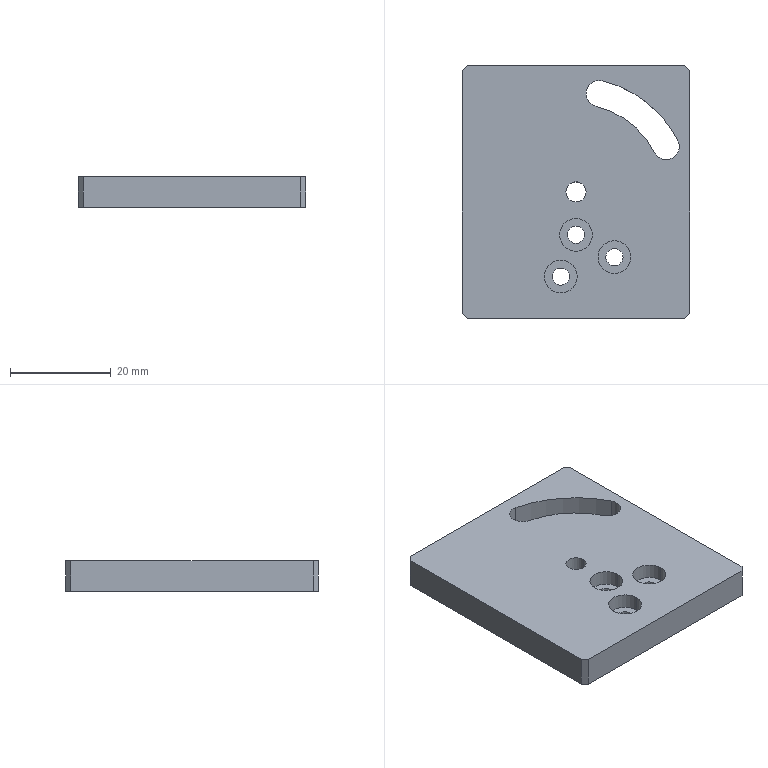Part | NX | features BREP 1 | 1 solid | 32 faces | box 45 x 50 x 6 mm | volume 12360 mm3 | cylinder 19 | plane 13 | commonest cylinder face diameters 3.4 x6 6.5 x6 5.2 x3 4 x2 34.8 x1 45.2 x1
STEP:
#1=CARTESIAN_POINT('',(-3.25,-8.489,3.));
#2=VERTEX_POINT('',#1);
#3=CARTESIAN_POINT('',(3.25,-8.489,3.));
#4=VERTEX_POINT('',#3);
#5=CARTESIAN_POINT('',(0.,-8.489,3.));
#6=DIRECTION('',(0.,0.,1.));
#7=DIRECTION('',(1.,0.,0.));
#8=AXIS2_PLACEMENT_3D('',#5,#6,#7);
#9=CIRCLE('',#8,3.25);
#10=EDGE_CURVE('',#2,#4,#9,.T.);
#11=ORIENTED_EDGE('',*,*,#10,.F.);
#12=CARTESIAN_POINT('',(-3.25,-8.489,6.));
#13=VERTEX_POINT('',#12);
#14=CARTESIAN_POINT('',(-3.25,-8.489,6.));
#15=DIRECTION('',(0.,0.,1.));
#16=VECTOR('',#15,1000.);
#17=LINE('',#14,#16);
#18=EDGE_CURVE('',#13,#2,#17,.F.);
#19=ORIENTED_EDGE('',*,*,#18,.F.);
#20=CARTESIAN_POINT('',(3.25,-8.489,6.));
#21=VERTEX_POINT('',#20);
#22=CARTESIAN_POINT('',(0.,-8.489,6.));
#23=DIRECTION('',(0.,0.,1.));
#24=DIRECTION('',(1.,0.,0.));
#25=AXIS2_PLACEMENT_3D('',#22,#23,#24);
#26=CIRCLE('',#25,3.25);
#27=EDGE_CURVE('',#13,#21,#26,.T.);
#28=ORIENTED_EDGE('',*,*,#27,.T.);
#29=CARTESIAN_POINT('',(3.25,-8.489,6.));
#30=DIRECTION('',(0.,0.,1.));
#31=VECTOR('',#30,1000.);
#32=LINE('',#29,#31);
#33=EDGE_CURVE('',#21,#4,#32,.F.);
#34=ORIENTED_EDGE('',*,*,#33,.T.);
#35=EDGE_LOOP('',(#11,#19,#28,#34));
#36=FACE_BOUND('',#35,.T.);
#37=CARTESIAN_POINT('',(0.,-8.489,6.));
#38=DIRECTION('',(0.,0.,1.));
#39=DIRECTION('',(1.,0.,0.));
#40=AXIS2_PLACEMENT_3D('',#37,#38,#39);
#41=CYLINDRICAL_SURFACE('',#40,3.25);
#42=ADVANCED_FACE('',(#36),#41,.F.);
#43=CARTESIAN_POINT('',(-1.7,-8.489,0.));
#44=VERTEX_POINT('',#43);
#45=CARTESIAN_POINT('',(1.7,-8.489,0.));
#46=VERTEX_POINT('',#45);
#47=CARTESIAN_POINT('',(0.,-8.489,0.));
#48=DIRECTION('',(0.,0.,1.));
#49=DIRECTION('',(1.,0.,0.));
#50=AXIS2_PLACEMENT_3D('',#47,#48,#49);
#51=CIRCLE('',#50,1.7);
#52=EDGE_CURVE('',#44,#46,#51,.T.);
#53=ORIENTED_EDGE('',*,*,#52,.F.);
#54=CARTESIAN_POINT('',(-1.7,-8.489,3.));
#55=VERTEX_POINT('',#54);
#56=CARTESIAN_POINT('',(-1.7,-8.489,6.));
#57=DIRECTION('',(0.,0.,1.));
#58=VECTOR('',#57,1000.);
#59=LINE('',#56,#58);
#60=EDGE_CURVE('',#55,#44,#59,.F.);
#61=ORIENTED_EDGE('',*,*,#60,.F.);
#62=CARTESIAN_POINT('',(1.7,-8.489,3.));
#63=VERTEX_POINT('',#62);
#64=CARTESIAN_POINT('',(0.,-8.489,3.));
#65=DIRECTION('',(0.,0.,1.));
#66=DIRECTION('',(1.,0.,0.));
#67=AXIS2_PLACEMENT_3D('',#64,#65,#66);
#68=CIRCLE('',#67,1.7);
#69=EDGE_CURVE('',#55,#63,#68,.T.);
#70=ORIENTED_EDGE('',*,*,#69,.T.);
#71=CARTESIAN_POINT('',(1.7,-8.489,6.));
#72=DIRECTION('',(0.,0.,1.));
#73=VECTOR('',#72,1000.);
#74=LINE('',#71,#73);
#75=EDGE_CURVE('',#63,#46,#74,.F.);
#76=ORIENTED_EDGE('',*,*,#75,.T.);
#77=EDGE_LOOP('',(#53,#61,#70,#76));
#78=FACE_BOUND('',#77,.T.);
#79=CARTESIAN_POINT('',(0.,-8.489,6.));
#80=DIRECTION('',(0.,0.,1.));
#81=DIRECTION('',(1.,0.,0.));
#82=AXIS2_PLACEMENT_3D('',#79,#80,#81);
#83=CYLINDRICAL_SURFACE('',#82,1.7);
#84=ADVANCED_FACE('',(#78),#83,.F.);
#85=CARTESIAN_POINT('',(-6.26,-16.759,3.));
#86=VERTEX_POINT('',#85);
#87=CARTESIAN_POINT('',(0.2402,-16.759,3.));
#88=VERTEX_POINT('',#87);
#89=CARTESIAN_POINT('',(-3.01,-16.759,3.));
#90=DIRECTION('',(0.,0.,1.));
#91=DIRECTION('',(1.,0.,0.));
#92=AXIS2_PLACEMENT_3D('',#89,#90,#91);
#93=CIRCLE('',#92,3.25);
#94=EDGE_CURVE('',#86,#88,#93,.T.);
#95=ORIENTED_EDGE('',*,*,#94,.F.);
#96=CARTESIAN_POINT('',(-6.26,-16.759,6.));
#97=VERTEX_POINT('',#96);
#98=CARTESIAN_POINT('',(-6.26,-16.759,6.));
#99=DIRECTION('',(0.,0.,1.));
#100=VECTOR('',#99,1000.);
#101=LINE('',#98,#100);
#102=EDGE_CURVE('',#97,#86,#101,.F.);
#103=ORIENTED_EDGE('',*,*,#102,.F.);
#104=CARTESIAN_POINT('',(0.2402,-16.759,6.));
#105=VERTEX_POINT('',#104);
#106=CARTESIAN_POINT('',(-3.01,-16.759,6.));
#107=DIRECTION('',(0.,0.,1.));
#108=DIRECTION('',(1.,0.,0.));
#109=AXIS2_PLACEMENT_3D('',#106,#107,#108);
#110=CIRCLE('',#109,3.25);
#111=EDGE_CURVE('',#97,#105,#110,.T.);
#112=ORIENTED_EDGE('',*,*,#111,.T.);
#113=CARTESIAN_POINT('',(0.2402,-16.759,6.));
#114=DIRECTION('',(0.,0.,1.));
#115=VECTOR('',#114,1000.);
#116=LINE('',#113,#115);
#117=EDGE_CURVE('',#105,#88,#116,.F.);
#118=ORIENTED_EDGE('',*,*,#117,.T.);
#119=EDGE_LOOP('',(#95,#103,#112,#118));
#120=FACE_BOUND('',#119,.T.);
#121=CARTESIAN_POINT('',(-3.01,-16.759,6.));
#122=DIRECTION('',(0.,0.,1.));
#123=DIRECTION('',(1.,0.,0.));
#124=AXIS2_PLACEMENT_3D('',#121,#122,#123);
#125=CYLINDRICAL_SURFACE('',#124,3.25);
#126=ADVANCED_FACE('',(#120),#125,.F.);
#127=CARTESIAN_POINT('',(-4.71,-16.759,0.));
#128=VERTEX_POINT('',#127);
#129=CARTESIAN_POINT('',(-1.31,-16.759,0.));
#130=VERTEX_POINT('',#129);
#131=CARTESIAN_POINT('',(-3.01,-16.759,0.));
#132=DIRECTION('',(0.,0.,1.));
#133=DIRECTION('',(1.,0.,0.));
#134=AXIS2_PLACEMENT_3D('',#131,#132,#133);
#135=CIRCLE('',#134,1.7);
#136=EDGE_CURVE('',#128,#130,#135,.T.);
#137=ORIENTED_EDGE('',*,*,#136,.F.);
#138=CARTESIAN_POINT('',(-4.71,-16.759,3.));
#139=VERTEX_POINT('',#138);
#140=CARTESIAN_POINT('',(-4.71,-16.759,6.));
#141=DIRECTION('',(0.,0.,1.));
#142=VECTOR('',#141,1000.);
#143=LINE('',#140,#142);
#144=EDGE_CURVE('',#139,#128,#143,.F.);
#145=ORIENTED_EDGE('',*,*,#144,.F.);
#146=CARTESIAN_POINT('',(-1.31,-16.759,3.));
#147=VERTEX_POINT('',#146);
#148=CARTESIAN_POINT('',(-3.01,-16.759,3.));
#149=DIRECTION('',(0.,0.,1.));
#150=DIRECTION('',(1.,0.,0.));
#151=AXIS2_PLACEMENT_3D('',#148,#149,#150);
#152=CIRCLE('',#151,1.7);
#153=EDGE_CURVE('',#139,#147,#152,.T.);
#154=ORIENTED_EDGE('',*,*,#153,.T.);
#155=CARTESIAN_POINT('',(-1.31,-16.759,6.));
#156=DIRECTION('',(0.,0.,1.));
#157=VECTOR('',#156,1000.);
#158=LINE('',#155,#157);
#159=EDGE_CURVE('',#147,#130,#158,.F.);
#160=ORIENTED_EDGE('',*,*,#159,.T.);
#161=EDGE_LOOP('',(#137,#145,#154,#160));
#162=FACE_BOUND('',#161,.T.);
#163=CARTESIAN_POINT('',(-3.01,-16.759,6.));
#164=DIRECTION('',(0.,0.,1.));
#165=DIRECTION('',(1.,0.,0.));
#166=AXIS2_PLACEMENT_3D('',#163,#164,#165);
#167=CYLINDRICAL_SURFACE('',#166,1.7);
#168=ADVANCED_FACE('',(#162),#167,.F.);
#169=CARTESIAN_POINT('',(4.362,-12.904,3.));
#170=VERTEX_POINT('',#169);
#171=CARTESIAN_POINT('',(10.862,-12.904,3.));
#172=VERTEX_POINT('',#171);
#173=CARTESIAN_POINT('',(7.612,-12.904,3.));
#174=DIRECTION('',(0.,0.,1.));
#175=DIRECTION('',(1.,0.,0.));
#176=AXIS2_PLACEMENT_3D('',#173,#174,#175);
#177=CIRCLE('',#176,3.25);
#178=EDGE_CURVE('',#170,#172,#177,.T.);
#179=ORIENTED_EDGE('',*,*,#178,.F.);
#180=CARTESIAN_POINT('',(4.362,-12.904,6.));
#181=VERTEX_POINT('',#180);
#182=CARTESIAN_POINT('',(4.362,-12.904,6.));
#183=DIRECTION('',(0.,0.,1.));
#184=VECTOR('',#183,1000.);
#185=LINE('',#182,#184);
#186=EDGE_CURVE('',#181,#170,#185,.F.);
#187=ORIENTED_EDGE('',*,*,#186,.F.);
#188=CARTESIAN_POINT('',(10.862,-12.904,6.));
#189=VERTEX_POINT('',#188);
#190=CARTESIAN_POINT('',(7.612,-12.904,6.));
#191=DIRECTION('',(0.,0.,1.));
#192=DIRECTION('',(1.,0.,0.));
#193=AXIS2_PLACEMENT_3D('',#190,#191,#192);
#194=CIRCLE('',#193,3.25);
#195=EDGE_CURVE('',#181,#189,#194,.T.);
#196=ORIENTED_EDGE('',*,*,#195,.T.);
#197=CARTESIAN_POINT('',(10.862,-12.904,6.));
#198=DIRECTION('',(0.,0.,1.));
#199=VECTOR('',#198,1000.);
#200=LINE('',#197,#199);
#201=EDGE_CURVE('',#189,#172,#200,.F.);
#202=ORIENTED_EDGE('',*,*,#201,.T.);
#203=EDGE_LOOP('',(#179,#187,#196,#202));
#204=FACE_BOUND('',#203,.T.);
#205=CARTESIAN_POINT('',(7.612,-12.904,6.));
#206=DIRECTION('',(0.,0.,1.));
#207=DIRECTION('',(1.,0.,0.));
#208=AXIS2_PLACEMENT_3D('',#205,#206,#207);
#209=CYLINDRICAL_SURFACE('',#208,3.25);
#210=ADVANCED_FACE('',(#204),#209,.F.);
#211=CARTESIAN_POINT('',(5.912,-12.904,0.));
#212=VERTEX_POINT('',#211);
#213=CARTESIAN_POINT('',(9.312,-12.904,0.));
#214=VERTEX_POINT('',#213);
#215=CARTESIAN_POINT('',(7.612,-12.904,0.));
#216=DIRECTION('',(0.,0.,1.));
#217=DIRECTION('',(1.,0.,0.));
#218=AXIS2_PLACEMENT_3D('',#215,#216,#217);
#219=CIRCLE('',#218,1.7);
#220=EDGE_CURVE('',#212,#214,#219,.T.);
#221=ORIENTED_EDGE('',*,*,#220,.F.);
#222=CARTESIAN_POINT('',(5.912,-12.904,3.));
#223=VERTEX_POINT('',#222);
#224=CARTESIAN_POINT('',(5.912,-12.904,6.));
#225=DIRECTION('',(0.,0.,1.));
#226=VECTOR('',#225,1000.);
#227=LINE('',#224,#226);
#228=EDGE_CURVE('',#223,#212,#227,.F.);
#229=ORIENTED_EDGE('',*,*,#228,.F.);
#230=CARTESIAN_POINT('',(9.312,-12.904,3.));
#231=VERTEX_POINT('',#230);
#232=CARTESIAN_POINT('',(7.612,-12.904,3.));
#233=DIRECTION('',(0.,0.,1.));
#234=DIRECTION('',(1.,0.,0.));
#235=AXIS2_PLACEMENT_3D('',#232,#233,#234);
#236=CIRCLE('',#235,1.7);
#237=EDGE_CURVE('',#223,#231,#236,.T.);
#238=ORIENTED_EDGE('',*,*,#237,.T.);
#239=CARTESIAN_POINT('',(9.312,-12.904,6.));
#240=DIRECTION('',(0.,0.,1.));
#241=VECTOR('',#240,1000.);
#242=LINE('',#239,#241);
#243=EDGE_CURVE('',#231,#214,#242,.F.);
#244=ORIENTED_EDGE('',*,*,#243,.T.);
#245=EDGE_LOOP('',(#221,#229,#238,#244));
#246=FACE_BOUND('',#245,.T.);
#247=CARTESIAN_POINT('',(7.612,-12.904,6.));
#248=DIRECTION('',(0.,0.,1.));
#249=DIRECTION('',(1.,0.,0.));
#250=AXIS2_PLACEMENT_3D('',#247,#248,#249);
#251=CYLINDRICAL_SURFACE('',#250,1.7);
#252=ADVANCED_FACE('',(#246),#251,.F.);
#253=CARTESIAN_POINT('',(5.182,21.998,6.));
#254=VERTEX_POINT('',#253);
#255=CARTESIAN_POINT('',(1.986,19.467,6.));
#256=VERTEX_POINT('',#255);
#257=CARTESIAN_POINT('',(4.586,19.467,6.));
#258=DIRECTION('',(0.,0.,1.));
#259=DIRECTION('',(1.,0.,0.));
#260=AXIS2_PLACEMENT_3D('',#257,#258,#259);
#261=CIRCLE('',#260,2.6);
#262=EDGE_CURVE('',#254,#256,#261,.T.);
#263=ORIENTED_EDGE('',*,*,#262,.T.);
#264=CARTESIAN_POINT('',(1.986,19.467,0.));
#265=VERTEX_POINT('',#264);
#266=CARTESIAN_POINT('',(1.986,19.467,10.));
#267=DIRECTION('',(0.,0.,-1.));
#268=VECTOR('',#267,1000.);
#269=LINE('',#266,#268);
#270=EDGE_CURVE('',#256,#265,#269,.T.);
#271=ORIENTED_EDGE('',*,*,#270,.T.);
#272=CARTESIAN_POINT('',(5.182,21.998,0.));
#273=VERTEX_POINT('',#272);
#274=CARTESIAN_POINT('',(4.586,19.467,0.));
#275=DIRECTION('',(0.,0.,-1.));
#276=DIRECTION('',(-1.,0.,0.));
#277=AXIS2_PLACEMENT_3D('',#274,#275,#276);
#278=CIRCLE('',#277,2.6);
#279=EDGE_CURVE('',#265,#273,#278,.T.);
#280=ORIENTED_EDGE('',*,*,#279,.T.);
#281=CARTESIAN_POINT('',(5.182,21.998,10.));
#282=DIRECTION('',(0.,0.,-1.));
#283=VECTOR('',#282,1000.);
#284=LINE('',#281,#283);
#285=EDGE_CURVE('',#254,#273,#284,.T.);
#286=ORIENTED_EDGE('',*,*,#285,.F.);
#287=EDGE_LOOP('',(#263,#271,#280,#286));
#288=FACE_BOUND('',#287,.T.);
#289=CARTESIAN_POINT('',(4.586,19.467,10.));
#290=DIRECTION('',(0.,0.,-1.));
#291=DIRECTION('',(-1.,0.,0.));
#292=AXIS2_PLACEMENT_3D('',#289,#290,#291);
#293=CYLINDRICAL_SURFACE('',#292,2.6);
#294=ADVANCED_FACE('',(#288),#293,.F.);
#295=CARTESIAN_POINT('',(-2.,0.,6.));
#296=VERTEX_POINT('',#295);
#297=CARTESIAN_POINT('',(2.,0.,6.));
#298=VERTEX_POINT('',#297);
#299=CARTESIAN_POINT('',(0.,0.,6.));
#300=DIRECTION('',(0.,0.,1.));
#301=DIRECTION('',(1.,0.,0.));
#302=AXIS2_PLACEMENT_3D('',#299,#300,#301);
#303=CIRCLE('',#302,2.);
#304=EDGE_CURVE('',#296,#298,#303,.T.);
#305=ORIENTED_EDGE('',*,*,#304,.T.);
#306=CARTESIAN_POINT('',(2.,0.,0.));
#307=VERTEX_POINT('',#306);
#308=CARTESIAN_POINT('',(2.,0.,10.));
#309=DIRECTION('',(0.,0.,-1.));
#310=VECTOR('',#309,1000.);
#311=LINE('',#308,#310);
#312=EDGE_CURVE('',#298,#307,#311,.T.);
#313=ORIENTED_EDGE('',*,*,#312,.T.);
#314=CARTESIAN_POINT('',(-2.,0.,0.));
#315=VERTEX_POINT('',#314);
#316=CARTESIAN_POINT('',(0.,0.,0.));
#317=DIRECTION('',(0.,0.,-1.));
#318=DIRECTION('',(-1.,0.,0.));
#319=AXIS2_PLACEMENT_3D('',#316,#317,#318);
#320=CIRCLE('',#319,2.);
#321=EDGE_CURVE('',#307,#315,#320,.T.);
#322=ORIENTED_EDGE('',*,*,#321,.T.);
#323=CARTESIAN_POINT('',(-2.,0.,10.));
#324=DIRECTION('',(0.,0.,-1.));
#325=VECTOR('',#324,1000.);
#326=LINE('',#323,#325);
#327=EDGE_CURVE('',#296,#315,#326,.T.);
#328=ORIENTED_EDGE('',*,*,#327,.F.);
#329=EDGE_LOOP('',(#305,#313,#322,#328));
#330=FACE_BOUND('',#329,.T.);
#331=CARTESIAN_POINT('',(0.,0.,10.));
#332=DIRECTION('',(0.,0.,-1.));
#333=DIRECTION('',(-1.,0.,0.));
#334=AXIS2_PLACEMENT_3D('',#331,#332,#333);
#335=CYLINDRICAL_SURFACE('',#334,2.);
#336=ADVANCED_FACE('',(#330),#335,.F.);
#337=CARTESIAN_POINT('',(22.5,-24.,6.));
#338=VERTEX_POINT('',#337);
#339=CARTESIAN_POINT('',(22.5,24.,6.));
#340=VERTEX_POINT('',#339);
#341=CARTESIAN_POINT('',(22.5,25.,6.));
#342=DIRECTION('',(0.,1.,0.));
#343=VECTOR('',#342,1000.);
#344=LINE('',#341,#343);
#345=EDGE_CURVE('',#338,#340,#344,.T.);
#346=ORIENTED_EDGE('',*,*,#345,.F.);
#347=CARTESIAN_POINT('',(22.5,-24.,0.));
#348=VERTEX_POINT('',#347);
#349=CARTESIAN_POINT('',(22.5,-24.,6.));
#350=DIRECTION('',(0.,0.,-1.));
#351=VECTOR('',#350,1000.);
#352=LINE('',#349,#351);
#353=EDGE_CURVE('',#338,#348,#352,.T.);
#354=ORIENTED_EDGE('',*,*,#353,.T.);
#355=CARTESIAN_POINT('',(22.5,24.,0.));
#356=VERTEX_POINT('',#355);
#357=CARTESIAN_POINT('',(22.5,25.,0.));
#358=DIRECTION('',(0.,1.,0.));
#359=VECTOR('',#358,1000.);
#360=LINE('',#357,#359);
#361=EDGE_CURVE('',#348,#356,#360,.T.);
#362=ORIENTED_EDGE('',*,*,#361,.T.);
#363=CARTESIAN_POINT('',(22.5,24.,6.));
#364=DIRECTION('',(0.,0.,1.));
#365=VECTOR('',#364,1000.);
#366=LINE('',#363,#365);
#367=EDGE_CURVE('',#356,#340,#366,.T.);
#368=ORIENTED_EDGE('',*,*,#367,.T.);
#369=EDGE_LOOP('',(#346,#354,#362,#368));
#370=FACE_BOUND('',#369,.T.);
#371=CARTESIAN_POINT('',(22.5,25.,6.));
#372=DIRECTION('',(-1.,0.,0.));
#373=DIRECTION('',(0.,1.,0.));
#374=AXIS2_PLACEMENT_3D('',#371,#372,#373);
#375=PLANE('',#374);
#376=ADVANCED_FACE('',(#370),#375,.F.);
#377=CARTESIAN_POINT('',(21.5,25.,0.));
#378=VERTEX_POINT('',#377);
#379=CARTESIAN_POINT('',(-21.5,25.,0.));
#380=VERTEX_POINT('',#379);
#381=CARTESIAN_POINT('',(-22.5,25.,0.));
#382=DIRECTION('',(-1.,0.,0.));
#383=VECTOR('',#382,1000.);
#384=LINE('',#381,#383);
#385=EDGE_CURVE('',#378,#380,#384,.T.);
#386=ORIENTED_EDGE('',*,*,#385,.T.);
#387=CARTESIAN_POINT('',(-21.5,25.,6.));
#388=VERTEX_POINT('',#387);
#389=CARTESIAN_POINT('',(-21.5,25.,6.));
#390=DIRECTION('',(0.,0.,1.));
#391=VECTOR('',#390,1000.);
#392=LINE('',#389,#391);
#393=EDGE_CURVE('',#380,#388,#392,.T.);
#394=ORIENTED_EDGE('',*,*,#393,.T.);
#395=CARTESIAN_POINT('',(21.5,25.,6.));
#396=VERTEX_POINT('',#395);
#397=CARTESIAN_POINT('',(-22.5,25.,6.));
#398=DIRECTION('',(-1.,0.,0.));
#399=VECTOR('',#398,1000.);
#400=LINE('',#397,#399);
#401=EDGE_CURVE('',#396,#388,#400,.T.);
#402=ORIENTED_EDGE('',*,*,#401,.F.);
#403=CARTESIAN_POINT('',(21.5,25.,6.));
#404=DIRECTION('',(0.,0.,-1.));
#405=VECTOR('',#404,1000.);
#406=LINE('',#403,#405);
#407=EDGE_CURVE('',#396,#378,#406,.T.);
#408=ORIENTED_EDGE('',*,*,#407,.T.);
#409=EDGE_LOOP('',(#386,#394,#402,#408));
#410=FACE_BOUND('',#409,.T.);
#411=CARTESIAN_POINT('',(-22.5,25.,6.));
#412=DIRECTION('',(0.,-1.,0.));
#413=DIRECTION('',(0.,0.,-1.));
#414=AXIS2_PLACEMENT_3D('',#411,#412,#413);
#415=PLANE('',#414);
#416=ADVANCED_FACE('',(#410),#415,.F.);
#417=CARTESIAN_POINT('',(-22.5,24.,0.));
#418=VERTEX_POINT('',#417);
#419=CARTESIAN_POINT('',(-22.5,-24.,0.));
#420=VERTEX_POINT('',#419);
#421=CARTESIAN_POINT('',(-22.5,25.,0.));
#422=DIRECTION('',(0.,-1.,0.));
#423=VECTOR('',#422,1000.);
#424=LINE('',#421,#423);
#425=EDGE_CURVE('',#418,#420,#424,.T.);
#426=ORIENTED_EDGE('',*,*,#425,.T.);
#427=CARTESIAN_POINT('',(-22.5,-24.,6.));
#428=VERTEX_POINT('',#427);
#429=CARTESIAN_POINT('',(-22.5,-24.,6.));
#430=DIRECTION('',(0.,0.,1.));
#431=VECTOR('',#430,1000.);
#432=LINE('',#429,#431);
#433=EDGE_CURVE('',#420,#428,#432,.T.);
#434=ORIENTED_EDGE('',*,*,#433,.T.);
#435=CARTESIAN_POINT('',(-22.5,24.,6.));
#436=VERTEX_POINT('',#435);
#437=CARTESIAN_POINT('',(-22.5,25.,6.));
#438=DIRECTION('',(0.,-1.,0.));
#439=VECTOR('',#438,1000.);
#440=LINE('',#437,#439);
#441=EDGE_CURVE('',#436,#428,#440,.T.);
#442=ORIENTED_EDGE('',*,*,#441,.F.);
#443=CARTESIAN_POINT('',(-22.5,24.,6.));
#444=DIRECTION('',(0.,0.,-1.));
#445=VECTOR('',#444,1000.);
#446=LINE('',#443,#445);
#447=EDGE_CURVE('',#436,#418,#446,.T.);
#448=ORIENTED_EDGE('',*,*,#447,.T.);
#449=EDGE_LOOP('',(#426,#434,#442,#448));
#450=FACE_BOUND('',#449,.T.);
#451=CARTESIAN_POINT('',(-22.5,25.,6.));
#452=DIRECTION('',(1.,0.,0.));
#453=DIRECTION('',(0.,1.,0.));
#454=AXIS2_PLACEMENT_3D('',#451,#452,#453);
#455=PLANE('',#454);
#456=ADVANCED_FACE('',(#450),#455,.F.);
#457=CARTESIAN_POINT('',(-21.5,-25.,6.));
#458=VERTEX_POINT('',#457);
#459=CARTESIAN_POINT('',(21.5,-25.,6.));
#460=VERTEX_POINT('',#459);
#461=CARTESIAN_POINT('',(-22.5,-25.,6.));
#462=DIRECTION('',(1.,0.,0.));
#463=VECTOR('',#462,1000.);
#464=LINE('',#461,#463);
#465=EDGE_CURVE('',#458,#460,#464,.T.);
#466=ORIENTED_EDGE('',*,*,#465,.F.);
#467=CARTESIAN_POINT('',(-21.5,-25.,0.));
#468=VERTEX_POINT('',#467);
#469=CARTESIAN_POINT('',(-21.5,-25.,6.));
#470=DIRECTION('',(0.,0.,-1.));
#471=VECTOR('',#470,1000.);
#472=LINE('',#469,#471);
#473=EDGE_CURVE('',#458,#468,#472,.T.);
#474=ORIENTED_EDGE('',*,*,#473,.T.);
#475=CARTESIAN_POINT('',(21.5,-25.,0.));
#476=VERTEX_POINT('',#475);
#477=CARTESIAN_POINT('',(-22.5,-25.,0.));
#478=DIRECTION('',(1.,0.,0.));
#479=VECTOR('',#478,1000.);
#480=LINE('',#477,#479);
#481=EDGE_CURVE('',#468,#476,#480,.T.);
#482=ORIENTED_EDGE('',*,*,#481,.T.);
#483=CARTESIAN_POINT('',(21.5,-25.,6.));
#484=DIRECTION('',(0.,0.,1.));
#485=VECTOR('',#484,1000.);
#486=LINE('',#483,#485);
#487=EDGE_CURVE('',#476,#460,#486,.T.);
#488=ORIENTED_EDGE('',*,*,#487,.T.);
#489=EDGE_LOOP('',(#466,#474,#482,#488));
#490=FACE_BOUND('',#489,.T.);
#491=CARTESIAN_POINT('',(-22.5,-25.,6.));
#492=DIRECTION('',(0.,1.,0.));
#493=DIRECTION('',(1.,0.,0.));
#494=AXIS2_PLACEMENT_3D('',#491,#492,#493);
#495=PLANE('',#494);
#496=ADVANCED_FACE('',(#490),#495,.F.);
#497=ORIENTED_EDGE('',*,*,#441,.T.);
#498=CARTESIAN_POINT('',(-23.25,-23.25,6.));
#499=DIRECTION('',(0.7071,-0.7071,0.));
#500=VECTOR('',#499,1000.);
#501=LINE('',#498,#500);
#502=EDGE_CURVE('',#428,#458,#501,.T.);
#503=ORIENTED_EDGE('',*,*,#502,.T.);
#504=ORIENTED_EDGE('',*,*,#465,.T.);
#505=CARTESIAN_POINT('',(23.25,-23.25,6.));
#506=DIRECTION('',(0.7071,0.7071,0.));
#507=VECTOR('',#506,1000.);
#508=LINE('',#505,#507);
#509=EDGE_CURVE('',#460,#338,#508,.T.);
#510=ORIENTED_EDGE('',*,*,#509,.T.);
#511=ORIENTED_EDGE('',*,*,#345,.T.);
#512=CARTESIAN_POINT('',(23.25,23.25,6.));
#513=DIRECTION('',(-0.7071,0.7071,0.));
#514=VECTOR('',#513,1000.);
#515=LINE('',#512,#514);
#516=EDGE_CURVE('',#340,#396,#515,.T.);
#517=ORIENTED_EDGE('',*,*,#516,.T.);
#518=ORIENTED_EDGE('',*,*,#401,.T.);
#519=CARTESIAN_POINT('',(-23.25,23.25,6.));
#520=DIRECTION('',(-0.7071,-0.7071,0.));
#521=VECTOR('',#520,1000.);
#522=LINE('',#519,#521);
#523=EDGE_CURVE('',#388,#436,#522,.T.);
#524=ORIENTED_EDGE('',*,*,#523,.T.);
#525=EDGE_LOOP('',(#497,#503,#504,#510,#511,#517,#518,#524));
#526=FACE_BOUND('',#525,.T.);
#527=CARTESIAN_POINT('',(0.,-8.489,6.));
#528=DIRECTION('',(0.,0.,1.));
#529=DIRECTION('',(1.,0.,0.));
#530=AXIS2_PLACEMENT_3D('',#527,#528,#529);
#531=CIRCLE('',#530,3.25);
#532=EDGE_CURVE('',#21,#13,#531,.T.);
#533=ORIENTED_EDGE('',*,*,#532,.F.);
#534=ORIENTED_EDGE('',*,*,#27,.F.);
#535=EDGE_LOOP('',(#533,#534));
#536=FACE_BOUND('',#535,.T.);
#537=CARTESIAN_POINT('',(-3.01,-16.759,6.));
#538=DIRECTION('',(0.,0.,1.));
#539=DIRECTION('',(1.,0.,0.));
#540=AXIS2_PLACEMENT_3D('',#537,#538,#539);
#541=CIRCLE('',#540,3.25);
#542=EDGE_CURVE('',#105,#97,#541,.T.);
#543=ORIENTED_EDGE('',*,*,#542,.F.);
#544=ORIENTED_EDGE('',*,*,#111,.F.);
#545=EDGE_LOOP('',(#543,#544));
#546=FACE_BOUND('',#545,.T.);
#547=CARTESIAN_POINT('',(7.612,-12.904,6.));
#548=DIRECTION('',(0.,0.,1.));
#549=DIRECTION('',(1.,0.,0.));
#550=AXIS2_PLACEMENT_3D('',#547,#548,#549);
#551=CIRCLE('',#550,3.25);
#552=EDGE_CURVE('',#189,#181,#551,.T.);
#553=ORIENTED_EDGE('',*,*,#552,.F.);
#554=ORIENTED_EDGE('',*,*,#195,.F.);
#555=EDGE_LOOP('',(#553,#554));
#556=FACE_BOUND('',#555,.T.);
#557=ORIENTED_EDGE('',*,*,#262,.F.);
#558=CARTESIAN_POINT('',(20.182,10.17,6.));
#559=VERTEX_POINT('',#558);
#560=CARTESIAN_POINT('',(0.,0.,6.));
#561=DIRECTION('',(0.,0.,1.));
#562=DIRECTION('',(1.,0.,0.));
#563=AXIS2_PLACEMENT_3D('',#560,#561,#562);
#564=CIRCLE('',#563,22.6);
#565=EDGE_CURVE('',#559,#254,#564,.T.);
#566=ORIENTED_EDGE('',*,*,#565,.F.);
#567=CARTESIAN_POINT('',(15.539,7.83,6.));
#568=VERTEX_POINT('',#567);
#569=CARTESIAN_POINT('',(17.861,9.,6.));
#570=DIRECTION('',(0.,0.,1.));
#571=DIRECTION('',(1.,0.,0.));
#572=AXIS2_PLACEMENT_3D('',#569,#570,#571);
#573=CIRCLE('',#572,2.6);
#574=EDGE_CURVE('',#568,#559,#573,.T.);
#575=ORIENTED_EDGE('',*,*,#574,.F.);
#576=CARTESIAN_POINT('',(3.99,16.936,6.));
#577=VERTEX_POINT('',#576);
#578=CARTESIAN_POINT('',(0.,0.,6.));
#579=DIRECTION('',(0.,0.,-1.));
#580=DIRECTION('',(1.,0.,0.));
#581=AXIS2_PLACEMENT_3D('',#578,#579,#580);
#582=CIRCLE('',#581,17.4);
#583=EDGE_CURVE('',#577,#568,#582,.T.);
#584=ORIENTED_EDGE('',*,*,#583,.F.);
#585=CARTESIAN_POINT('',(4.586,19.467,6.));
#586=DIRECTION('',(0.,0.,1.));
#587=DIRECTION('',(1.,0.,0.));
#588=AXIS2_PLACEMENT_3D('',#585,#586,#587);
#589=CIRCLE('',#588,2.6);
#590=EDGE_CURVE('',#256,#577,#589,.T.);
#591=ORIENTED_EDGE('',*,*,#590,.F.);
#592=EDGE_LOOP('',(#557,#566,#575,#584,#591));
#593=FACE_BOUND('',#592,.T.);
#594=ORIENTED_EDGE('',*,*,#304,.F.);
#595=CARTESIAN_POINT('',(0.,0.,6.));
#596=DIRECTION('',(0.,0.,1.));
#597=DIRECTION('',(1.,0.,0.));
#598=AXIS2_PLACEMENT_3D('',#595,#596,#597);
#599=CIRCLE('',#598,2.);
#600=EDGE_CURVE('',#298,#296,#599,.T.);
#601=ORIENTED_EDGE('',*,*,#600,.F.);
#602=EDGE_LOOP('',(#594,#601));
#603=FACE_BOUND('',#602,.T.);
#604=CARTESIAN_POINT('',(0.,0.,6.));
#605=DIRECTION('',(0.,0.,1.));
#606=DIRECTION('',(1.,0.,0.));
#607=AXIS2_PLACEMENT_3D('',#604,#605,#606);
#608=PLANE('',#607);
#609=ADVANCED_FACE('',(#526,#536,#546,#556,#593,#603),#608,.T.);
#610=ORIENTED_EDGE('',*,*,#481,.F.);
#611=CARTESIAN_POINT('',(-21.5,-25.,0.));
#612=DIRECTION('',(-0.7071,0.7071,0.));
#613=VECTOR('',#612,1000.);
#614=LINE('',#611,#613);
#615=EDGE_CURVE('',#468,#420,#614,.T.);
#616=ORIENTED_EDGE('',*,*,#615,.T.);
#617=ORIENTED_EDGE('',*,*,#425,.F.);
#618=CARTESIAN_POINT('',(-22.5,24.,0.));
#619=DIRECTION('',(0.7071,0.7071,0.));
#620=VECTOR('',#619,1000.);
#621=LINE('',#618,#620);
#622=EDGE_CURVE('',#418,#380,#621,.T.);
#623=ORIENTED_EDGE('',*,*,#622,.T.);
#624=ORIENTED_EDGE('',*,*,#385,.F.);
#625=CARTESIAN_POINT('',(21.5,25.,0.));
#626=DIRECTION('',(0.7071,-0.7071,0.));
#627=VECTOR('',#626,1000.);
#628=LINE('',#625,#627);
#629=EDGE_CURVE('',#378,#356,#628,.T.);
#630=ORIENTED_EDGE('',*,*,#629,.T.);
#631=ORIENTED_EDGE('',*,*,#361,.F.);
#632=CARTESIAN_POINT('',(22.5,-24.,0.));
#633=DIRECTION('',(-0.7071,-0.7071,0.));
#634=VECTOR('',#633,1000.);
#635=LINE('',#632,#634);
#636=EDGE_CURVE('',#348,#476,#635,.T.);
#637=ORIENTED_EDGE('',*,*,#636,.T.);
#638=EDGE_LOOP('',(#610,#616,#617,#623,#624,#630,#631,#637));
#639=FACE_BOUND('',#638,.T.);
#640=CARTESIAN_POINT('',(0.,-8.489,0.));
#641=DIRECTION('',(0.,0.,1.));
#642=DIRECTION('',(1.,0.,0.));
#643=AXIS2_PLACEMENT_3D('',#640,#641,#642);
#644=CIRCLE('',#643,1.7);
#645=EDGE_CURVE('',#46,#44,#644,.T.);
#646=ORIENTED_EDGE('',*,*,#645,.T.);
#647=ORIENTED_EDGE('',*,*,#52,.T.);
#648=EDGE_LOOP('',(#646,#647));
#649=FACE_BOUND('',#648,.T.);
#650=CARTESIAN_POINT('',(-3.01,-16.759,0.));
#651=DIRECTION('',(0.,0.,1.));
#652=DIRECTION('',(1.,0.,0.));
#653=AXIS2_PLACEMENT_3D('',#650,#651,#652);
#654=CIRCLE('',#653,1.7);
#655=EDGE_CURVE('',#130,#128,#654,.T.);
#656=ORIENTED_EDGE('',*,*,#655,.T.);
#657=ORIENTED_EDGE('',*,*,#136,.T.);
#658=EDGE_LOOP('',(#656,#657));
#659=FACE_BOUND('',#658,.T.);
#660=CARTESIAN_POINT('',(7.612,-12.904,0.));
#661=DIRECTION('',(0.,0.,1.));
#662=DIRECTION('',(1.,0.,0.));
#663=AXIS2_PLACEMENT_3D('',#660,#661,#662);
#664=CIRCLE('',#663,1.7);
#665=EDGE_CURVE('',#214,#212,#664,.T.);
#666=ORIENTED_EDGE('',*,*,#665,.T.);
#667=ORIENTED_EDGE('',*,*,#220,.T.);
#668=EDGE_LOOP('',(#666,#667));
#669=FACE_BOUND('',#668,.T.);
#670=CARTESIAN_POINT('',(20.182,10.17,0.));
#671=VERTEX_POINT('',#670);
#672=CARTESIAN_POINT('',(0.,0.,0.));
#673=DIRECTION('',(0.,0.,-1.));
#674=DIRECTION('',(-1.,0.,0.));
#675=AXIS2_PLACEMENT_3D('',#672,#673,#674);
#676=CIRCLE('',#675,22.6);
#677=EDGE_CURVE('',#273,#671,#676,.T.);
#678=ORIENTED_EDGE('',*,*,#677,.F.);
#679=ORIENTED_EDGE('',*,*,#279,.F.);
#680=CARTESIAN_POINT('',(3.99,16.936,0.));
#681=VERTEX_POINT('',#680);
#682=CARTESIAN_POINT('',(4.586,19.467,0.));
#683=DIRECTION('',(0.,0.,-1.));
#684=DIRECTION('',(-1.,0.,0.));
#685=AXIS2_PLACEMENT_3D('',#682,#683,#684);
#686=CIRCLE('',#685,2.6);
#687=EDGE_CURVE('',#681,#265,#686,.T.);
#688=ORIENTED_EDGE('',*,*,#687,.F.);
#689=CARTESIAN_POINT('',(15.539,7.83,0.));
#690=VERTEX_POINT('',#689);
#691=CARTESIAN_POINT('',(0.,0.,0.));
#692=DIRECTION('',(0.,0.,1.));
#693=DIRECTION('',(-1.,0.,0.));
#694=AXIS2_PLACEMENT_3D('',#691,#692,#693);
#695=CIRCLE('',#694,17.4);
#696=EDGE_CURVE('',#690,#681,#695,.T.);
#697=ORIENTED_EDGE('',*,*,#696,.F.);
#698=CARTESIAN_POINT('',(17.861,9.,0.));
#699=DIRECTION('',(0.,0.,-1.));
#700=DIRECTION('',(-1.,0.,0.));
#701=AXIS2_PLACEMENT_3D('',#698,#699,#700);
#702=CIRCLE('',#701,2.6);
#703=EDGE_CURVE('',#671,#690,#702,.T.);
#704=ORIENTED_EDGE('',*,*,#703,.F.);
#705=EDGE_LOOP('',(#678,#679,#688,#697,#704));
#706=FACE_BOUND('',#705,.T.);
#707=CARTESIAN_POINT('',(0.,0.,0.));
#708=DIRECTION('',(0.,0.,-1.));
#709=DIRECTION('',(-1.,0.,0.));
#710=AXIS2_PLACEMENT_3D('',#707,#708,#709);
#711=CIRCLE('',#710,2.);
#712=EDGE_CURVE('',#315,#307,#711,.T.);
#713=ORIENTED_EDGE('',*,*,#712,.F.);
#714=ORIENTED_EDGE('',*,*,#321,.F.);
#715=EDGE_LOOP('',(#713,#714));
#716=FACE_BOUND('',#715,.T.);
#717=CARTESIAN_POINT('',(0.,0.,0.));
#718=DIRECTION('',(0.,0.,1.));
#719=DIRECTION('',(1.,0.,0.));
#720=AXIS2_PLACEMENT_3D('',#717,#718,#719);
#721=PLANE('',#720);
#722=ADVANCED_FACE('',(#639,#649,#659,#669,#706,#716),#721,.F.);
#723=ORIENTED_EDGE('',*,*,#502,.F.);
#724=ORIENTED_EDGE('',*,*,#433,.F.);
#725=ORIENTED_EDGE('',*,*,#615,.F.);
#726=ORIENTED_EDGE('',*,*,#473,.F.);
#727=EDGE_LOOP('',(#723,#724,#725,#726));
#728=FACE_BOUND('',#727,.T.);
#729=CARTESIAN_POINT('',(-21.5,-25.,6.));
#730=DIRECTION('',(0.7071,0.7071,0.));
#731=DIRECTION('',(0.,0.,-1.));
#732=AXIS2_PLACEMENT_3D('',#729,#730,#731);
#733=PLANE('',#732);
#734=ADVANCED_FACE('',(#728),#733,.F.);
#735=ORIENTED_EDGE('',*,*,#509,.F.);
#736=ORIENTED_EDGE('',*,*,#487,.F.);
#737=ORIENTED_EDGE('',*,*,#636,.F.);
#738=ORIENTED_EDGE('',*,*,#353,.F.);
#739=EDGE_LOOP('',(#735,#736,#737,#738));
#740=FACE_BOUND('',#739,.T.);
#741=CARTESIAN_POINT('',(22.5,-24.,6.));
#742=DIRECTION('',(-0.7071,0.7071,0.));
#743=DIRECTION('',(0.,0.,1.));
#744=AXIS2_PLACEMENT_3D('',#741,#742,#743);
#745=PLANE('',#744);
#746=ADVANCED_FACE('',(#740),#745,.F.);
#747=ORIENTED_EDGE('',*,*,#523,.F.);
#748=ORIENTED_EDGE('',*,*,#393,.F.);
#749=ORIENTED_EDGE('',*,*,#622,.F.);
#750=ORIENTED_EDGE('',*,*,#447,.F.);
#751=EDGE_LOOP('',(#747,#748,#749,#750));
#752=FACE_BOUND('',#751,.T.);
#753=CARTESIAN_POINT('',(-22.5,24.,6.));
#754=DIRECTION('',(0.7071,-0.7071,0.));
#755=DIRECTION('',(0.,0.,-1.));
#756=AXIS2_PLACEMENT_3D('',#753,#754,#755);
#757=PLANE('',#756);
#758=ADVANCED_FACE('',(#752),#757,.F.);
#759=ORIENTED_EDGE('',*,*,#516,.F.);
#760=ORIENTED_EDGE('',*,*,#367,.F.);
#761=ORIENTED_EDGE('',*,*,#629,.F.);
#762=ORIENTED_EDGE('',*,*,#407,.F.);
#763=EDGE_LOOP('',(#759,#760,#761,#762));
#764=FACE_BOUND('',#763,.T.);
#765=CARTESIAN_POINT('',(21.5,25.,6.));
#766=DIRECTION('',(-0.7071,-0.7071,0.));
#767=DIRECTION('',(-0.7071,0.7071,0.));
#768=AXIS2_PLACEMENT_3D('',#765,#766,#767);
#769=PLANE('',#768);
#770=ADVANCED_FACE('',(#764),#769,.F.);
#771=ORIENTED_EDGE('',*,*,#312,.F.);
#772=ORIENTED_EDGE('',*,*,#600,.T.);
#773=ORIENTED_EDGE('',*,*,#327,.T.);
#774=ORIENTED_EDGE('',*,*,#712,.T.);
#775=EDGE_LOOP('',(#771,#772,#773,#774));
#776=FACE_BOUND('',#775,.T.);
#777=CARTESIAN_POINT('',(0.,0.,10.));
#778=DIRECTION('',(0.,0.,-1.));
#779=DIRECTION('',(-1.,0.,0.));
#780=AXIS2_PLACEMENT_3D('',#777,#778,#779);
#781=CYLINDRICAL_SURFACE('',#780,2.);
#782=ADVANCED_FACE('',(#776),#781,.F.);
#783=ORIENTED_EDGE('',*,*,#270,.F.);
#784=ORIENTED_EDGE('',*,*,#590,.T.);
#785=CARTESIAN_POINT('',(3.99,16.936,10.));
#786=DIRECTION('',(0.,0.,-1.));
#787=VECTOR('',#786,1000.);
#788=LINE('',#785,#787);
#789=EDGE_CURVE('',#577,#681,#788,.T.);
#790=ORIENTED_EDGE('',*,*,#789,.T.);
#791=ORIENTED_EDGE('',*,*,#687,.T.);
#792=EDGE_LOOP('',(#783,#784,#790,#791));
#793=FACE_BOUND('',#792,.T.);
#794=CARTESIAN_POINT('',(4.586,19.467,10.));
#795=DIRECTION('',(0.,0.,-1.));
#796=DIRECTION('',(-1.,0.,0.));
#797=AXIS2_PLACEMENT_3D('',#794,#795,#796);
#798=CYLINDRICAL_SURFACE('',#797,2.6);
#799=ADVANCED_FACE('',(#793),#798,.F.);
#800=ORIENTED_EDGE('',*,*,#583,.T.);
#801=CARTESIAN_POINT('',(15.539,7.83,10.));
#802=DIRECTION('',(0.,0.,-1.));
#803=VECTOR('',#802,1000.);
#804=LINE('',#801,#803);
#805=EDGE_CURVE('',#568,#690,#804,.T.);
#806=ORIENTED_EDGE('',*,*,#805,.T.);
#807=ORIENTED_EDGE('',*,*,#696,.T.);
#808=ORIENTED_EDGE('',*,*,#789,.F.);
#809=EDGE_LOOP('',(#800,#806,#807,#808));
#810=FACE_BOUND('',#809,.T.);
#811=CARTESIAN_POINT('',(0.,0.,10.));
#812=DIRECTION('',(0.,0.,-1.));
#813=DIRECTION('',(-1.,0.,0.));
#814=AXIS2_PLACEMENT_3D('',#811,#812,#813);
#815=CYLINDRICAL_SURFACE('',#814,17.4);
#816=ADVANCED_FACE('',(#810),#815,.T.);
#817=ORIENTED_EDGE('',*,*,#574,.T.);
#818=CARTESIAN_POINT('',(20.182,10.17,10.));
#819=DIRECTION('',(0.,0.,-1.));
#820=VECTOR('',#819,1000.);
#821=LINE('',#818,#820);
#822=EDGE_CURVE('',#559,#671,#821,.T.);
#823=ORIENTED_EDGE('',*,*,#822,.T.);
#824=ORIENTED_EDGE('',*,*,#703,.T.);
#825=ORIENTED_EDGE('',*,*,#805,.F.);
#826=EDGE_LOOP('',(#817,#823,#824,#825));
#827=FACE_BOUND('',#826,.T.);
#828=CARTESIAN_POINT('',(17.861,9.,10.));
#829=DIRECTION('',(0.,0.,-1.));
#830=DIRECTION('',(-1.,0.,0.));
#831=AXIS2_PLACEMENT_3D('',#828,#829,#830);
#832=CYLINDRICAL_SURFACE('',#831,2.6);
#833=ADVANCED_FACE('',(#827),#832,.F.);
#834=ORIENTED_EDGE('',*,*,#565,.T.);
#835=ORIENTED_EDGE('',*,*,#285,.T.);
#836=ORIENTED_EDGE('',*,*,#677,.T.);
#837=ORIENTED_EDGE('',*,*,#822,.F.);
#838=EDGE_LOOP('',(#834,#835,#836,#837));
#839=FACE_BOUND('',#838,.T.);
#840=CARTESIAN_POINT('',(0.,0.,10.));
#841=DIRECTION('',(0.,0.,-1.));
#842=DIRECTION('',(-1.,0.,0.));
#843=AXIS2_PLACEMENT_3D('',#840,#841,#842);
#844=CYLINDRICAL_SURFACE('',#843,22.6);
#845=ADVANCED_FACE('',(#839),#844,.F.);
#846=ORIENTED_EDGE('',*,*,#228,.T.);
#847=ORIENTED_EDGE('',*,*,#665,.F.);
#848=ORIENTED_EDGE('',*,*,#243,.F.);
#849=CARTESIAN_POINT('',(7.612,-12.904,3.));
#850=DIRECTION('',(0.,0.,1.));
#851=DIRECTION('',(1.,0.,0.));
#852=AXIS2_PLACEMENT_3D('',#849,#850,#851);
#853=CIRCLE('',#852,1.7);
#854=EDGE_CURVE('',#231,#223,#853,.T.);
#855=ORIENTED_EDGE('',*,*,#854,.T.);
#856=EDGE_LOOP('',(#846,#847,#848,#855));
#857=FACE_BOUND('',#856,.T.);
#858=CARTESIAN_POINT('',(7.612,-12.904,6.));
#859=DIRECTION('',(0.,0.,1.));
#860=DIRECTION('',(1.,0.,0.));
#861=AXIS2_PLACEMENT_3D('',#858,#859,#860);
#862=CYLINDRICAL_SURFACE('',#861,1.7);
#863=ADVANCED_FACE('',(#857),#862,.F.);
#864=CARTESIAN_POINT('',(7.612,-12.904,3.));
#865=DIRECTION('',(0.,0.,1.));
#866=DIRECTION('',(1.,0.,0.));
#867=AXIS2_PLACEMENT_3D('',#864,#865,#866);
#868=CIRCLE('',#867,3.25);
#869=EDGE_CURVE('',#172,#170,#868,.T.);
#870=ORIENTED_EDGE('',*,*,#869,.T.);
#871=ORIENTED_EDGE('',*,*,#178,.T.);
#872=EDGE_LOOP('',(#870,#871));
#873=FACE_BOUND('',#872,.T.);
#874=ORIENTED_EDGE('',*,*,#854,.F.);
#875=ORIENTED_EDGE('',*,*,#237,.F.);
#876=EDGE_LOOP('',(#874,#875));
#877=FACE_BOUND('',#876,.T.);
#878=CARTESIAN_POINT('',(9.312,-12.904,3.));
#879=DIRECTION('',(0.,0.,-1.));
#880=DIRECTION('',(0.,-1.,0.));
#881=AXIS2_PLACEMENT_3D('',#878,#879,#880);
#882=PLANE('',#881);
#883=ADVANCED_FACE('',(#873,#877),#882,.F.);
#884=ORIENTED_EDGE('',*,*,#186,.T.);
#885=ORIENTED_EDGE('',*,*,#869,.F.);
#886=ORIENTED_EDGE('',*,*,#201,.F.);
#887=ORIENTED_EDGE('',*,*,#552,.T.);
#888=EDGE_LOOP('',(#884,#885,#886,#887));
#889=FACE_BOUND('',#888,.T.);
#890=CARTESIAN_POINT('',(7.612,-12.904,6.));
#891=DIRECTION('',(0.,0.,1.));
#892=DIRECTION('',(1.,0.,0.));
#893=AXIS2_PLACEMENT_3D('',#890,#891,#892);
#894=CYLINDRICAL_SURFACE('',#893,3.25);
#895=ADVANCED_FACE('',(#889),#894,.F.);
#896=ORIENTED_EDGE('',*,*,#144,.T.);
#897=ORIENTED_EDGE('',*,*,#655,.F.);
#898=ORIENTED_EDGE('',*,*,#159,.F.);
#899=CARTESIAN_POINT('',(-3.01,-16.759,3.));
#900=DIRECTION('',(0.,0.,1.));
#901=DIRECTION('',(1.,0.,0.));
#902=AXIS2_PLACEMENT_3D('',#899,#900,#901);
#903=CIRCLE('',#902,1.7);
#904=EDGE_CURVE('',#147,#139,#903,.T.);
#905=ORIENTED_EDGE('',*,*,#904,.T.);
#906=EDGE_LOOP('',(#896,#897,#898,#905));
#907=FACE_BOUND('',#906,.T.);
#908=CARTESIAN_POINT('',(-3.01,-16.759,6.));
#909=DIRECTION('',(0.,0.,1.));
#910=DIRECTION('',(1.,0.,0.));
#911=AXIS2_PLACEMENT_3D('',#908,#909,#910);
#912=CYLINDRICAL_SURFACE('',#911,1.7);
#913=ADVANCED_FACE('',(#907),#912,.F.);
#914=CARTESIAN_POINT('',(-3.01,-16.759,3.));
#915=DIRECTION('',(0.,0.,1.));
#916=DIRECTION('',(1.,0.,0.));
#917=AXIS2_PLACEMENT_3D('',#914,#915,#916);
#918=CIRCLE('',#917,3.25);
#919=EDGE_CURVE('',#88,#86,#918,.T.);
#920=ORIENTED_EDGE('',*,*,#919,.T.);
#921=ORIENTED_EDGE('',*,*,#94,.T.);
#922=EDGE_LOOP('',(#920,#921));
#923=FACE_BOUND('',#922,.T.);
#924=ORIENTED_EDGE('',*,*,#904,.F.);
#925=ORIENTED_EDGE('',*,*,#153,.F.);
#926=EDGE_LOOP('',(#924,#925));
#927=FACE_BOUND('',#926,.T.);
#928=CARTESIAN_POINT('',(-1.31,-16.759,3.));
#929=DIRECTION('',(0.,0.,-1.));
#930=DIRECTION('',(0.,-1.,0.));
#931=AXIS2_PLACEMENT_3D('',#928,#929,#930);
#932=PLANE('',#931);
#933=ADVANCED_FACE('',(#923,#927),#932,.F.);
#934=ORIENTED_EDGE('',*,*,#102,.T.);
#935=ORIENTED_EDGE('',*,*,#919,.F.);
#936=ORIENTED_EDGE('',*,*,#117,.F.);
#937=ORIENTED_EDGE('',*,*,#542,.T.);
#938=EDGE_LOOP('',(#934,#935,#936,#937));
#939=FACE_BOUND('',#938,.T.);
#940=CARTESIAN_POINT('',(-3.01,-16.759,6.));
#941=DIRECTION('',(0.,0.,1.));
#942=DIRECTION('',(1.,0.,0.));
#943=AXIS2_PLACEMENT_3D('',#940,#941,#942);
#944=CYLINDRICAL_SURFACE('',#943,3.25);
#945=ADVANCED_FACE('',(#939),#944,.F.);
#946=ORIENTED_EDGE('',*,*,#60,.T.);
#947=ORIENTED_EDGE('',*,*,#645,.F.);
#948=ORIENTED_EDGE('',*,*,#75,.F.);
#949=CARTESIAN_POINT('',(0.,-8.489,3.));
#950=DIRECTION('',(0.,0.,1.));
#951=DIRECTION('',(1.,0.,0.));
#952=AXIS2_PLACEMENT_3D('',#949,#950,#951);
#953=CIRCLE('',#952,1.7);
#954=EDGE_CURVE('',#63,#55,#953,.T.);
#955=ORIENTED_EDGE('',*,*,#954,.T.);
#956=EDGE_LOOP('',(#946,#947,#948,#955));
#957=FACE_BOUND('',#956,.T.);
#958=CARTESIAN_POINT('',(0.,-8.489,6.));
#959=DIRECTION('',(0.,0.,1.));
#960=DIRECTION('',(1.,0.,0.));
#961=AXIS2_PLACEMENT_3D('',#958,#959,#960);
#962=CYLINDRICAL_SURFACE('',#961,1.7);
#963=ADVANCED_FACE('',(#957),#962,.F.);
#964=CARTESIAN_POINT('',(0.,-8.489,3.));
#965=DIRECTION('',(0.,0.,1.));
#966=DIRECTION('',(1.,0.,0.));
#967=AXIS2_PLACEMENT_3D('',#964,#965,#966);
#968=CIRCLE('',#967,3.25);
#969=EDGE_CURVE('',#4,#2,#968,.T.);
#970=ORIENTED_EDGE('',*,*,#969,.T.);
#971=ORIENTED_EDGE('',*,*,#10,.T.);
#972=EDGE_LOOP('',(#970,#971));
#973=FACE_BOUND('',#972,.T.);
#974=ORIENTED_EDGE('',*,*,#954,.F.);
#975=ORIENTED_EDGE('',*,*,#69,.F.);
#976=EDGE_LOOP('',(#974,#975));
#977=FACE_BOUND('',#976,.T.);
#978=CARTESIAN_POINT('',(1.7,-8.489,3.));
#979=DIRECTION('',(0.,0.,-1.));
#980=DIRECTION('',(0.,-1.,0.));
#981=AXIS2_PLACEMENT_3D('',#978,#979,#980);
#982=PLANE('',#981);
#983=ADVANCED_FACE('',(#973,#977),#982,.F.);
#984=ORIENTED_EDGE('',*,*,#18,.T.);
#985=ORIENTED_EDGE('',*,*,#969,.F.);
#986=ORIENTED_EDGE('',*,*,#33,.F.);
#987=ORIENTED_EDGE('',*,*,#532,.T.);
#988=EDGE_LOOP('',(#984,#985,#986,#987));
#989=FACE_BOUND('',#988,.T.);
#990=CARTESIAN_POINT('',(0.,-8.489,6.));
#991=DIRECTION('',(0.,0.,1.));
#992=DIRECTION('',(1.,0.,0.));
#993=AXIS2_PLACEMENT_3D('',#990,#991,#992);
#994=CYLINDRICAL_SURFACE('',#993,3.25);
#995=ADVANCED_FACE('',(#989),#994,.F.);
#996=CLOSED_SHELL('',(#42,#84,#126,#168,#210,#252,#294,#336,#376,#416,#456,#496,#609,#722,#734,#746,#758,#770,#782,#799,#816,#833,#845,#863,#883,#895,#913,#933,#945,#963,#983,#995));
#997=MANIFOLD_SOLID_BREP('',#996);
#998=(LENGTH_UNIT()NAMED_UNIT(*)SI_UNIT(.MILLI.,.METRE.));
#999=UNCERTAINTY_MEASURE_WITH_UNIT(LENGTH_MEASURE(0.00001),#998,'','');
#1000=(NAMED_UNIT(*)PLANE_ANGLE_UNIT()SI_UNIT($,.RADIAN.));
#1001=(NAMED_UNIT(*)SI_UNIT($,.STERADIAN.)SOLID_ANGLE_UNIT());
#1002=(GEOMETRIC_REPRESENTATION_CONTEXT(3)GLOBAL_UNCERTAINTY_ASSIGNED_CONTEXT((#999))GLOBAL_UNIT_ASSIGNED_CONTEXT((#998,#1000,#1001))REPRESENTATION_CONTEXT('',''));
#1003=ADVANCED_BREP_SHAPE_REPRESENTATION('',(#997),#1002);